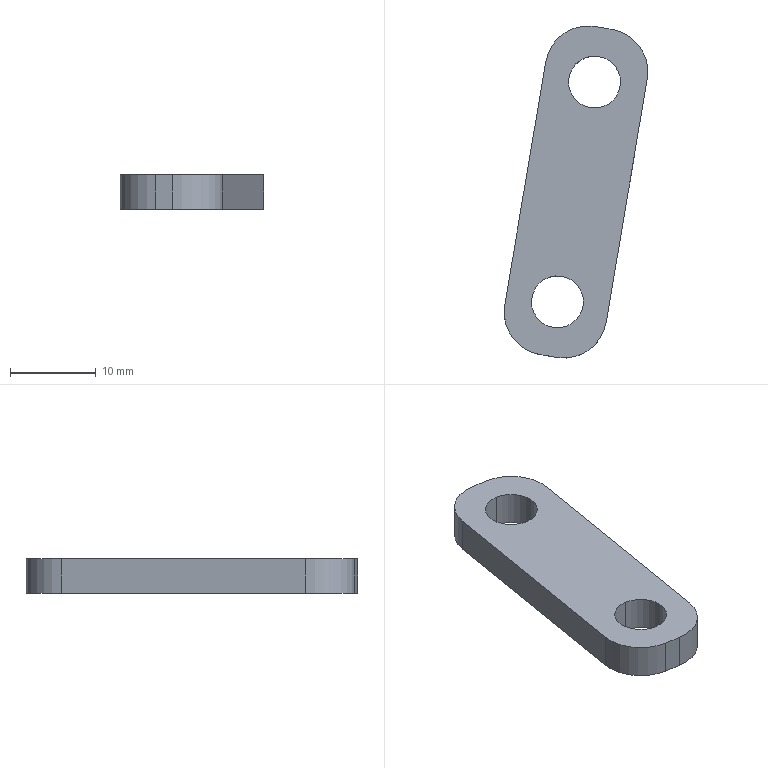Part | NX | features BREP 1 | 1 solid | 14 faces | box 16.766 x 38.731 x 4 mm | volume 1546 mm3 | cylinder 8 | plane 6 | commonest cylinder face diameters 6.06 x4 10 x4
STEP:
#1=CARTESIAN_POINT('',(-15.824,146.625,10.));
#2=VERTEX_POINT('',#1);
#3=CARTESIAN_POINT('',(-16.832,140.65,10.));
#4=VERTEX_POINT('',#3);
#5=CARTESIAN_POINT('',(-16.328,143.638,10.));
#6=DIRECTION('',(0.,0.,-1.));
#7=DIRECTION('',(-0.1665,-0.986,0.));
#8=AXIS2_PLACEMENT_3D('',#5,#6,#7);
#9=CIRCLE('',#8,3.03);
#10=EDGE_CURVE('',#2,#4,#9,.T.);
#11=ORIENTED_EDGE('',*,*,#10,.T.);
#12=CARTESIAN_POINT('',(-16.832,140.65,14.));
#13=VERTEX_POINT('',#12);
#14=CARTESIAN_POINT('',(-16.832,140.65,10.));
#15=DIRECTION('',(0.,0.,-1.));
#16=VECTOR('',#15,1000.);
#17=LINE('',#14,#16);
#18=EDGE_CURVE('',#13,#4,#17,.T.);
#19=ORIENTED_EDGE('',*,*,#18,.F.);
#20=CARTESIAN_POINT('',(-15.824,146.625,14.));
#21=VERTEX_POINT('',#20);
#22=CARTESIAN_POINT('',(-16.328,143.638,14.));
#23=DIRECTION('',(0.,0.,-1.));
#24=DIRECTION('',(-0.1665,-0.986,0.));
#25=AXIS2_PLACEMENT_3D('',#22,#23,#24);
#26=CIRCLE('',#25,3.03);
#27=EDGE_CURVE('',#21,#13,#26,.T.);
#28=ORIENTED_EDGE('',*,*,#27,.F.);
#29=CARTESIAN_POINT('',(-15.824,146.625,10.));
#30=DIRECTION('',(0.,0.,1.));
#31=VECTOR('',#30,1000.);
#32=LINE('',#29,#31);
#33=EDGE_CURVE('',#2,#21,#32,.T.);
#34=ORIENTED_EDGE('',*,*,#33,.F.);
#35=EDGE_LOOP('',(#11,#19,#28,#34));
#36=FACE_BOUND('',#35,.T.);
#37=CARTESIAN_POINT('',(-16.328,143.638,10.));
#38=DIRECTION('',(0.,0.,1.));
#39=DIRECTION('',(-0.1665,-0.986,0.));
#40=AXIS2_PLACEMENT_3D('',#37,#38,#39);
#41=CYLINDRICAL_SURFACE('',#40,3.03);
#42=ADVANCED_FACE('',(#36),#41,.F.);
#43=CARTESIAN_POINT('',(-11.496,172.263,10.));
#44=VERTEX_POINT('',#43);
#45=CARTESIAN_POINT('',(-12.504,166.287,10.));
#46=VERTEX_POINT('',#45);
#47=CARTESIAN_POINT('',(-12.,169.275,10.));
#48=DIRECTION('',(0.,0.,-1.));
#49=DIRECTION('',(-0.1665,-0.986,0.));
#50=AXIS2_PLACEMENT_3D('',#47,#48,#49);
#51=CIRCLE('',#50,3.03);
#52=EDGE_CURVE('',#44,#46,#51,.T.);
#53=ORIENTED_EDGE('',*,*,#52,.T.);
#54=CARTESIAN_POINT('',(-12.504,166.287,14.));
#55=VERTEX_POINT('',#54);
#56=CARTESIAN_POINT('',(-12.504,166.287,10.));
#57=DIRECTION('',(0.,0.,-1.));
#58=VECTOR('',#57,1000.);
#59=LINE('',#56,#58);
#60=EDGE_CURVE('',#55,#46,#59,.T.);
#61=ORIENTED_EDGE('',*,*,#60,.F.);
#62=CARTESIAN_POINT('',(-11.496,172.263,14.));
#63=VERTEX_POINT('',#62);
#64=CARTESIAN_POINT('',(-12.,169.275,14.));
#65=DIRECTION('',(0.,0.,-1.));
#66=DIRECTION('',(-0.1665,-0.986,0.));
#67=AXIS2_PLACEMENT_3D('',#64,#65,#66);
#68=CIRCLE('',#67,3.03);
#69=EDGE_CURVE('',#63,#55,#68,.T.);
#70=ORIENTED_EDGE('',*,*,#69,.F.);
#71=CARTESIAN_POINT('',(-11.496,172.263,10.));
#72=DIRECTION('',(0.,0.,1.));
#73=VECTOR('',#72,1000.);
#74=LINE('',#71,#73);
#75=EDGE_CURVE('',#44,#63,#74,.T.);
#76=ORIENTED_EDGE('',*,*,#75,.F.);
#77=EDGE_LOOP('',(#53,#61,#70,#76));
#78=FACE_BOUND('',#77,.T.);
#79=CARTESIAN_POINT('',(-12.,169.275,10.));
#80=DIRECTION('',(0.,0.,1.));
#81=DIRECTION('',(-0.1665,-0.986,0.));
#82=AXIS2_PLACEMENT_3D('',#79,#80,#81);
#83=CYLINDRICAL_SURFACE('',#82,3.03);
#84=ADVANCED_FACE('',(#78),#83,.F.);
#85=CARTESIAN_POINT('',(-16.407,137.161,10.));
#86=VERTEX_POINT('',#85);
#87=CARTESIAN_POINT('',(-18.379,137.494,10.));
#88=VERTEX_POINT('',#87);
#89=CARTESIAN_POINT('',(-11.477,136.328,10.));
#90=DIRECTION('',(-0.986,0.1665,0.));
#91=VECTOR('',#90,1000.);
#92=LINE('',#89,#91);
#93=EDGE_CURVE('',#86,#88,#92,.T.);
#94=ORIENTED_EDGE('',*,*,#93,.T.);
#95=CARTESIAN_POINT('',(-22.477,143.256,10.));
#96=VERTEX_POINT('',#95);
#97=CARTESIAN_POINT('',(-17.547,142.424,10.));
#98=DIRECTION('',(0.,0.,-1.));
#99=DIRECTION('',(0.1665,0.986,0.));
#100=AXIS2_PLACEMENT_3D('',#97,#98,#99);
#101=CIRCLE('',#100,5.);
#102=EDGE_CURVE('',#88,#96,#101,.T.);
#103=ORIENTED_EDGE('',*,*,#102,.T.);
#104=CARTESIAN_POINT('',(-17.683,171.654,10.));
#105=VERTEX_POINT('',#104);
#106=CARTESIAN_POINT('',(-23.31,138.326,10.));
#107=DIRECTION('',(0.1665,0.986,0.));
#108=VECTOR('',#107,1000.);
#109=LINE('',#106,#108);
#110=EDGE_CURVE('',#96,#105,#109,.T.);
#111=ORIENTED_EDGE('',*,*,#110,.T.);
#112=CARTESIAN_POINT('',(-11.921,175.752,10.));
#113=VERTEX_POINT('',#112);
#114=CARTESIAN_POINT('',(-12.753,170.822,10.));
#115=DIRECTION('',(0.,0.,-1.));
#116=DIRECTION('',(0.1665,0.986,0.));
#117=AXIS2_PLACEMENT_3D('',#114,#115,#116);
#118=CIRCLE('',#117,5.);
#119=EDGE_CURVE('',#105,#113,#118,.T.);
#120=ORIENTED_EDGE('',*,*,#119,.T.);
#121=CARTESIAN_POINT('',(-9.949,175.419,10.));
#122=VERTEX_POINT('',#121);
#123=CARTESIAN_POINT('',(-5.018,174.587,10.));
#124=DIRECTION('',(0.986,-0.1665,0.));
#125=VECTOR('',#124,1000.);
#126=LINE('',#123,#125);
#127=EDGE_CURVE('',#113,#122,#126,.T.);
#128=ORIENTED_EDGE('',*,*,#127,.T.);
#129=CARTESIAN_POINT('',(-5.851,169.657,10.));
#130=VERTEX_POINT('',#129);
#131=CARTESIAN_POINT('',(-10.781,170.489,10.));
#132=DIRECTION('',(0.,0.,-1.));
#133=DIRECTION('',(0.1665,0.986,0.));
#134=AXIS2_PLACEMENT_3D('',#131,#132,#133);
#135=CIRCLE('',#134,5.);
#136=EDGE_CURVE('',#122,#130,#135,.T.);
#137=ORIENTED_EDGE('',*,*,#136,.T.);
#138=CARTESIAN_POINT('',(-10.645,141.259,10.));
#139=VERTEX_POINT('',#138);
#140=CARTESIAN_POINT('',(-11.477,136.328,10.));
#141=DIRECTION('',(-0.1665,-0.986,0.));
#142=VECTOR('',#141,1000.);
#143=LINE('',#140,#142);
#144=EDGE_CURVE('',#130,#139,#143,.T.);
#145=ORIENTED_EDGE('',*,*,#144,.T.);
#146=CARTESIAN_POINT('',(-15.575,142.091,10.));
#147=DIRECTION('',(0.,0.,-1.));
#148=DIRECTION('',(0.1665,0.986,0.));
#149=AXIS2_PLACEMENT_3D('',#146,#147,#148);
#150=CIRCLE('',#149,5.);
#151=EDGE_CURVE('',#139,#86,#150,.T.);
#152=ORIENTED_EDGE('',*,*,#151,.T.);
#153=EDGE_LOOP('',(#94,#103,#111,#120,#128,#137,#145,#152));
#154=FACE_BOUND('',#153,.T.);
#155=ORIENTED_EDGE('',*,*,#52,.F.);
#156=CARTESIAN_POINT('',(-12.,169.275,10.));
#157=DIRECTION('',(0.,0.,-1.));
#158=DIRECTION('',(-0.1665,-0.986,0.));
#159=AXIS2_PLACEMENT_3D('',#156,#157,#158);
#160=CIRCLE('',#159,3.03);
#161=EDGE_CURVE('',#46,#44,#160,.T.);
#162=ORIENTED_EDGE('',*,*,#161,.F.);
#163=EDGE_LOOP('',(#155,#162));
#164=FACE_BOUND('',#163,.T.);
#165=ORIENTED_EDGE('',*,*,#10,.F.);
#166=CARTESIAN_POINT('',(-16.328,143.638,10.));
#167=DIRECTION('',(0.,0.,-1.));
#168=DIRECTION('',(-0.1665,-0.986,0.));
#169=AXIS2_PLACEMENT_3D('',#166,#167,#168);
#170=CIRCLE('',#169,3.03);
#171=EDGE_CURVE('',#4,#2,#170,.T.);
#172=ORIENTED_EDGE('',*,*,#171,.F.);
#173=EDGE_LOOP('',(#165,#172));
#174=FACE_BOUND('',#173,.T.);
#175=CARTESIAN_POINT('',(-11.477,136.328,10.));
#176=DIRECTION('',(0.,0.,1.));
#177=DIRECTION('',(-0.1665,-0.986,0.));
#178=AXIS2_PLACEMENT_3D('',#175,#176,#177);
#179=PLANE('',#178);
#180=ADVANCED_FACE('',(#154,#164,#174),#179,.F.);
#181=ORIENTED_EDGE('',*,*,#69,.T.);
#182=CARTESIAN_POINT('',(-12.,169.275,14.));
#183=DIRECTION('',(0.,0.,-1.));
#184=DIRECTION('',(-0.1665,-0.986,0.));
#185=AXIS2_PLACEMENT_3D('',#182,#183,#184);
#186=CIRCLE('',#185,3.03);
#187=EDGE_CURVE('',#55,#63,#186,.T.);
#188=ORIENTED_EDGE('',*,*,#187,.T.);
#189=EDGE_LOOP('',(#181,#188));
#190=FACE_BOUND('',#189,.T.);
#191=CARTESIAN_POINT('',(-22.477,143.256,14.));
#192=VERTEX_POINT('',#191);
#193=CARTESIAN_POINT('',(-17.683,171.654,14.));
#194=VERTEX_POINT('',#193);
#195=CARTESIAN_POINT('',(-23.31,138.326,14.));
#196=DIRECTION('',(0.1665,0.986,0.));
#197=VECTOR('',#196,1000.);
#198=LINE('',#195,#197);
#199=EDGE_CURVE('',#192,#194,#198,.T.);
#200=ORIENTED_EDGE('',*,*,#199,.F.);
#201=CARTESIAN_POINT('',(-18.379,137.494,14.));
#202=VERTEX_POINT('',#201);
#203=CARTESIAN_POINT('',(-17.547,142.424,14.));
#204=DIRECTION('',(0.,0.,1.));
#205=DIRECTION('',(0.1665,0.986,0.));
#206=AXIS2_PLACEMENT_3D('',#203,#204,#205);
#207=CIRCLE('',#206,5.);
#208=EDGE_CURVE('',#192,#202,#207,.T.);
#209=ORIENTED_EDGE('',*,*,#208,.T.);
#210=CARTESIAN_POINT('',(-16.407,137.161,14.));
#211=VERTEX_POINT('',#210);
#212=CARTESIAN_POINT('',(-11.477,136.328,14.));
#213=DIRECTION('',(-0.986,0.1665,0.));
#214=VECTOR('',#213,1000.);
#215=LINE('',#212,#214);
#216=EDGE_CURVE('',#211,#202,#215,.T.);
#217=ORIENTED_EDGE('',*,*,#216,.F.);
#218=CARTESIAN_POINT('',(-10.645,141.259,14.));
#219=VERTEX_POINT('',#218);
#220=CARTESIAN_POINT('',(-15.575,142.091,14.));
#221=DIRECTION('',(0.,0.,1.));
#222=DIRECTION('',(0.1665,0.986,0.));
#223=AXIS2_PLACEMENT_3D('',#220,#221,#222);
#224=CIRCLE('',#223,5.);
#225=EDGE_CURVE('',#211,#219,#224,.T.);
#226=ORIENTED_EDGE('',*,*,#225,.T.);
#227=CARTESIAN_POINT('',(-5.851,169.657,14.));
#228=VERTEX_POINT('',#227);
#229=CARTESIAN_POINT('',(-11.477,136.328,14.));
#230=DIRECTION('',(-0.1665,-0.986,0.));
#231=VECTOR('',#230,1000.);
#232=LINE('',#229,#231);
#233=EDGE_CURVE('',#228,#219,#232,.T.);
#234=ORIENTED_EDGE('',*,*,#233,.F.);
#235=CARTESIAN_POINT('',(-9.949,175.419,14.));
#236=VERTEX_POINT('',#235);
#237=CARTESIAN_POINT('',(-10.781,170.489,14.));
#238=DIRECTION('',(0.,0.,1.));
#239=DIRECTION('',(0.1665,0.986,0.));
#240=AXIS2_PLACEMENT_3D('',#237,#238,#239);
#241=CIRCLE('',#240,5.);
#242=EDGE_CURVE('',#228,#236,#241,.T.);
#243=ORIENTED_EDGE('',*,*,#242,.T.);
#244=CARTESIAN_POINT('',(-11.921,175.752,14.));
#245=VERTEX_POINT('',#244);
#246=CARTESIAN_POINT('',(-5.018,174.587,14.));
#247=DIRECTION('',(0.986,-0.1665,0.));
#248=VECTOR('',#247,1000.);
#249=LINE('',#246,#248);
#250=EDGE_CURVE('',#245,#236,#249,.T.);
#251=ORIENTED_EDGE('',*,*,#250,.F.);
#252=CARTESIAN_POINT('',(-12.753,170.822,14.));
#253=DIRECTION('',(0.,0.,1.));
#254=DIRECTION('',(0.1665,0.986,0.));
#255=AXIS2_PLACEMENT_3D('',#252,#253,#254);
#256=CIRCLE('',#255,5.);
#257=EDGE_CURVE('',#245,#194,#256,.T.);
#258=ORIENTED_EDGE('',*,*,#257,.T.);
#259=EDGE_LOOP('',(#200,#209,#217,#226,#234,#243,#251,#258));
#260=FACE_BOUND('',#259,.T.);
#261=ORIENTED_EDGE('',*,*,#27,.T.);
#262=CARTESIAN_POINT('',(-16.328,143.638,14.));
#263=DIRECTION('',(0.,0.,-1.));
#264=DIRECTION('',(-0.1665,-0.986,0.));
#265=AXIS2_PLACEMENT_3D('',#262,#263,#264);
#266=CIRCLE('',#265,3.03);
#267=EDGE_CURVE('',#13,#21,#266,.T.);
#268=ORIENTED_EDGE('',*,*,#267,.T.);
#269=EDGE_LOOP('',(#261,#268));
#270=FACE_BOUND('',#269,.T.);
#271=CARTESIAN_POINT('',(-11.477,136.328,14.));
#272=DIRECTION('',(0.,0.,1.));
#273=DIRECTION('',(-0.1665,-0.986,0.));
#274=AXIS2_PLACEMENT_3D('',#271,#272,#273);
#275=PLANE('',#274);
#276=ADVANCED_FACE('',(#190,#260,#270),#275,.T.);
#277=ORIENTED_EDGE('',*,*,#233,.T.);
#278=CARTESIAN_POINT('',(-10.645,141.259,10.));
#279=DIRECTION('',(0.,0.,-1.));
#280=VECTOR('',#279,1000.);
#281=LINE('',#278,#280);
#282=EDGE_CURVE('',#219,#139,#281,.T.);
#283=ORIENTED_EDGE('',*,*,#282,.T.);
#284=ORIENTED_EDGE('',*,*,#144,.F.);
#285=CARTESIAN_POINT('',(-5.851,169.657,10.));
#286=DIRECTION('',(0.,0.,1.));
#287=VECTOR('',#286,1000.);
#288=LINE('',#285,#287);
#289=EDGE_CURVE('',#130,#228,#288,.T.);
#290=ORIENTED_EDGE('',*,*,#289,.T.);
#291=EDGE_LOOP('',(#277,#283,#284,#290));
#292=FACE_BOUND('',#291,.T.);
#293=CARTESIAN_POINT('',(-11.477,136.328,10.));
#294=DIRECTION('',(-0.986,0.1665,0.));
#295=DIRECTION('',(-0.1665,-0.986,0.));
#296=AXIS2_PLACEMENT_3D('',#293,#294,#295);
#297=PLANE('',#296);
#298=ADVANCED_FACE('',(#292),#297,.F.);
#299=ORIENTED_EDGE('',*,*,#216,.T.);
#300=CARTESIAN_POINT('',(-18.379,137.494,10.));
#301=DIRECTION('',(0.,0.,-1.));
#302=VECTOR('',#301,1000.);
#303=LINE('',#300,#302);
#304=EDGE_CURVE('',#202,#88,#303,.T.);
#305=ORIENTED_EDGE('',*,*,#304,.T.);
#306=ORIENTED_EDGE('',*,*,#93,.F.);
#307=CARTESIAN_POINT('',(-16.407,137.161,10.));
#308=DIRECTION('',(0.,0.,1.));
#309=VECTOR('',#308,1000.);
#310=LINE('',#307,#309);
#311=EDGE_CURVE('',#86,#211,#310,.T.);
#312=ORIENTED_EDGE('',*,*,#311,.T.);
#313=EDGE_LOOP('',(#299,#305,#306,#312));
#314=FACE_BOUND('',#313,.T.);
#315=CARTESIAN_POINT('',(-11.477,136.328,10.));
#316=DIRECTION('',(0.1665,0.986,0.));
#317=DIRECTION('',(-0.986,0.1665,0.));
#318=AXIS2_PLACEMENT_3D('',#315,#316,#317);
#319=PLANE('',#318);
#320=ADVANCED_FACE('',(#314),#319,.F.);
#321=ORIENTED_EDGE('',*,*,#110,.F.);
#322=CARTESIAN_POINT('',(-22.477,143.256,10.));
#323=DIRECTION('',(0.,0.,1.));
#324=VECTOR('',#323,1000.);
#325=LINE('',#322,#324);
#326=EDGE_CURVE('',#96,#192,#325,.T.);
#327=ORIENTED_EDGE('',*,*,#326,.T.);
#328=ORIENTED_EDGE('',*,*,#199,.T.);
#329=CARTESIAN_POINT('',(-17.683,171.654,10.));
#330=DIRECTION('',(0.,0.,-1.));
#331=VECTOR('',#330,1000.);
#332=LINE('',#329,#331);
#333=EDGE_CURVE('',#194,#105,#332,.T.);
#334=ORIENTED_EDGE('',*,*,#333,.T.);
#335=EDGE_LOOP('',(#321,#327,#328,#334));
#336=FACE_BOUND('',#335,.T.);
#337=CARTESIAN_POINT('',(-23.31,138.326,10.));
#338=DIRECTION('',(0.986,-0.1665,0.));
#339=DIRECTION('',(0.1665,0.986,0.));
#340=AXIS2_PLACEMENT_3D('',#337,#338,#339);
#341=PLANE('',#340);
#342=ADVANCED_FACE('',(#336),#341,.F.);
#343=ORIENTED_EDGE('',*,*,#127,.F.);
#344=CARTESIAN_POINT('',(-11.921,175.752,10.));
#345=DIRECTION('',(0.,0.,1.));
#346=VECTOR('',#345,1000.);
#347=LINE('',#344,#346);
#348=EDGE_CURVE('',#113,#245,#347,.T.);
#349=ORIENTED_EDGE('',*,*,#348,.T.);
#350=ORIENTED_EDGE('',*,*,#250,.T.);
#351=CARTESIAN_POINT('',(-9.949,175.419,10.));
#352=DIRECTION('',(0.,0.,-1.));
#353=VECTOR('',#352,1000.);
#354=LINE('',#351,#353);
#355=EDGE_CURVE('',#236,#122,#354,.T.);
#356=ORIENTED_EDGE('',*,*,#355,.T.);
#357=EDGE_LOOP('',(#343,#349,#350,#356));
#358=FACE_BOUND('',#357,.T.);
#359=CARTESIAN_POINT('',(-5.018,174.587,10.));
#360=DIRECTION('',(-0.1665,-0.986,0.));
#361=DIRECTION('',(0.986,-0.1665,0.));
#362=AXIS2_PLACEMENT_3D('',#359,#360,#361);
#363=PLANE('',#362);
#364=ADVANCED_FACE('',(#358),#363,.F.);
#365=ORIENTED_EDGE('',*,*,#60,.T.);
#366=ORIENTED_EDGE('',*,*,#161,.T.);
#367=ORIENTED_EDGE('',*,*,#75,.T.);
#368=ORIENTED_EDGE('',*,*,#187,.F.);
#369=EDGE_LOOP('',(#365,#366,#367,#368));
#370=FACE_BOUND('',#369,.T.);
#371=CARTESIAN_POINT('',(-12.,169.275,10.));
#372=DIRECTION('',(0.,0.,1.));
#373=DIRECTION('',(-0.1665,-0.986,0.));
#374=AXIS2_PLACEMENT_3D('',#371,#372,#373);
#375=CYLINDRICAL_SURFACE('',#374,3.03);
#376=ADVANCED_FACE('',(#370),#375,.F.);
#377=ORIENTED_EDGE('',*,*,#18,.T.);
#378=ORIENTED_EDGE('',*,*,#171,.T.);
#379=ORIENTED_EDGE('',*,*,#33,.T.);
#380=ORIENTED_EDGE('',*,*,#267,.F.);
#381=EDGE_LOOP('',(#377,#378,#379,#380));
#382=FACE_BOUND('',#381,.T.);
#383=CARTESIAN_POINT('',(-16.328,143.638,10.));
#384=DIRECTION('',(0.,0.,1.));
#385=DIRECTION('',(-0.1665,-0.986,0.));
#386=AXIS2_PLACEMENT_3D('',#383,#384,#385);
#387=CYLINDRICAL_SURFACE('',#386,3.03);
#388=ADVANCED_FACE('',(#382),#387,.F.);
#389=ORIENTED_EDGE('',*,*,#102,.F.);
#390=ORIENTED_EDGE('',*,*,#304,.F.);
#391=ORIENTED_EDGE('',*,*,#208,.F.);
#392=ORIENTED_EDGE('',*,*,#326,.F.);
#393=EDGE_LOOP('',(#389,#390,#391,#392));
#394=FACE_BOUND('',#393,.T.);
#395=CARTESIAN_POINT('',(-17.547,142.424,10.));
#396=DIRECTION('',(0.,0.,1.));
#397=DIRECTION('',(-0.1665,-0.986,0.));
#398=AXIS2_PLACEMENT_3D('',#395,#396,#397);
#399=CYLINDRICAL_SURFACE('',#398,5.);
#400=ADVANCED_FACE('',(#394),#399,.T.);
#401=ORIENTED_EDGE('',*,*,#151,.F.);
#402=ORIENTED_EDGE('',*,*,#282,.F.);
#403=ORIENTED_EDGE('',*,*,#225,.F.);
#404=ORIENTED_EDGE('',*,*,#311,.F.);
#405=EDGE_LOOP('',(#401,#402,#403,#404));
#406=FACE_BOUND('',#405,.T.);
#407=CARTESIAN_POINT('',(-15.575,142.091,10.));
#408=DIRECTION('',(0.,0.,1.));
#409=DIRECTION('',(-0.1665,-0.986,0.));
#410=AXIS2_PLACEMENT_3D('',#407,#408,#409);
#411=CYLINDRICAL_SURFACE('',#410,5.);
#412=ADVANCED_FACE('',(#406),#411,.T.);
#413=ORIENTED_EDGE('',*,*,#119,.F.);
#414=ORIENTED_EDGE('',*,*,#333,.F.);
#415=ORIENTED_EDGE('',*,*,#257,.F.);
#416=ORIENTED_EDGE('',*,*,#348,.F.);
#417=EDGE_LOOP('',(#413,#414,#415,#416));
#418=FACE_BOUND('',#417,.T.);
#419=CARTESIAN_POINT('',(-12.753,170.822,10.));
#420=DIRECTION('',(0.,0.,1.));
#421=DIRECTION('',(-0.1665,-0.986,0.));
#422=AXIS2_PLACEMENT_3D('',#419,#420,#421);
#423=CYLINDRICAL_SURFACE('',#422,5.);
#424=ADVANCED_FACE('',(#418),#423,.T.);
#425=ORIENTED_EDGE('',*,*,#136,.F.);
#426=ORIENTED_EDGE('',*,*,#355,.F.);
#427=ORIENTED_EDGE('',*,*,#242,.F.);
#428=ORIENTED_EDGE('',*,*,#289,.F.);
#429=EDGE_LOOP('',(#425,#426,#427,#428));
#430=FACE_BOUND('',#429,.T.);
#431=CARTESIAN_POINT('',(-10.781,170.489,10.));
#432=DIRECTION('',(0.,0.,1.));
#433=DIRECTION('',(-0.1665,-0.986,0.));
#434=AXIS2_PLACEMENT_3D('',#431,#432,#433);
#435=CYLINDRICAL_SURFACE('',#434,5.);
#436=ADVANCED_FACE('',(#430),#435,.T.);
#437=CLOSED_SHELL('',(#42,#84,#180,#276,#298,#320,#342,#364,#376,#388,#400,#412,#424,#436));
#438=MANIFOLD_SOLID_BREP('',#437);
#439=(LENGTH_UNIT()NAMED_UNIT(*)SI_UNIT(.MILLI.,.METRE.));
#440=UNCERTAINTY_MEASURE_WITH_UNIT(LENGTH_MEASURE(0.00001),#439,'','');
#441=(NAMED_UNIT(*)PLANE_ANGLE_UNIT()SI_UNIT($,.RADIAN.));
#442=(NAMED_UNIT(*)SI_UNIT($,.STERADIAN.)SOLID_ANGLE_UNIT());
#443=(GEOMETRIC_REPRESENTATION_CONTEXT(3)GLOBAL_UNCERTAINTY_ASSIGNED_CONTEXT((#440))GLOBAL_UNIT_ASSIGNED_CONTEXT((#439,#441,#442))REPRESENTATION_CONTEXT('',''));
#444=ADVANCED_BREP_SHAPE_REPRESENTATION('',(#438),#443);